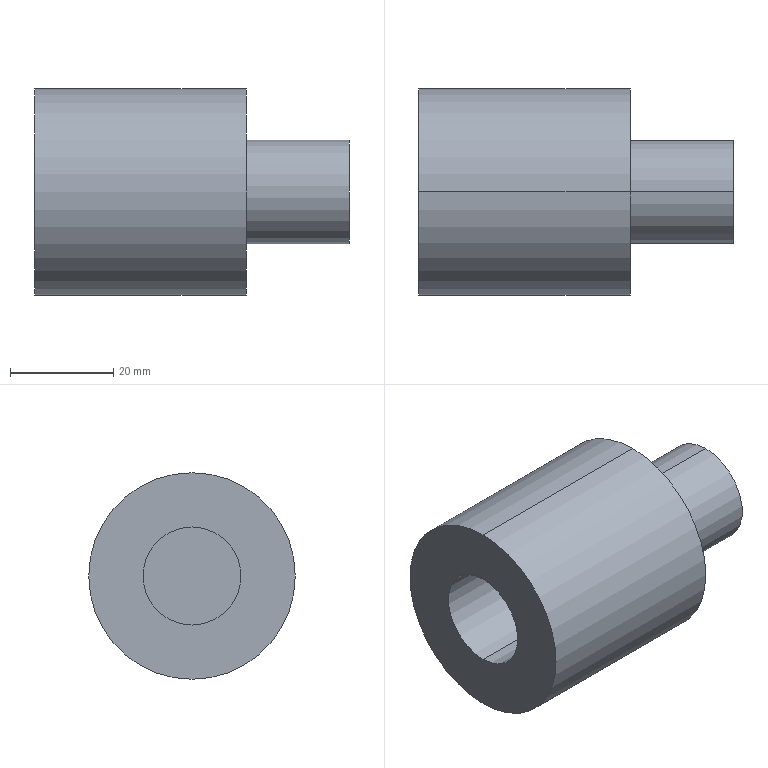Part | STEP file | _MAX100010001NA0_cupling2 | 1 solid | 10 faces | box 61 x 40 x 40 mm | volume 52985 mm3 | cylinder 6 | plane 4 | commonest cylinder face diameters 19 x2 20 x2 40 x2
STEP:
#1=CARTESIAN_POINT('',(504.,0.,20.));
#2=VERTEX_POINT('',#1);
#3=CARTESIAN_POINT('',(504.,0.,-20.));
#4=VERTEX_POINT('',#3);
#5=CARTESIAN_POINT('',(504.,0.,0.));
#6=DIRECTION('',(-1.,0.,0.));
#7=DIRECTION('',(0.,0.,1.));
#8=AXIS2_PLACEMENT_3D('',#5,#6,#7);
#9=CIRCLE('',#8,20.);
#10=EDGE_CURVE('',#2,#4,#9,.T.);
#11=ORIENTED_EDGE('',*,*,#10,.T.);
#12=CARTESIAN_POINT('',(463.,0.,-20.));
#13=VERTEX_POINT('',#12);
#14=CARTESIAN_POINT('',(524.,0.,-20.));
#15=DIRECTION('',(-1.,0.,0.));
#16=VECTOR('',#15,1000.);
#17=LINE('',#14,#16);
#18=EDGE_CURVE('',#4,#13,#17,.T.);
#19=ORIENTED_EDGE('',*,*,#18,.T.);
#20=CARTESIAN_POINT('',(463.,0.,20.));
#21=VERTEX_POINT('',#20);
#22=CARTESIAN_POINT('',(463.,0.,0.));
#23=DIRECTION('',(1.,0.,0.));
#24=DIRECTION('',(0.,0.,1.));
#25=AXIS2_PLACEMENT_3D('',#22,#23,#24);
#26=CIRCLE('',#25,20.);
#27=EDGE_CURVE('',#13,#21,#26,.T.);
#28=ORIENTED_EDGE('',*,*,#27,.T.);
#29=CARTESIAN_POINT('',(524.,0.,20.));
#30=DIRECTION('',(-1.,0.,0.));
#31=VECTOR('',#30,1000.);
#32=LINE('',#29,#31);
#33=EDGE_CURVE('',#2,#21,#32,.T.);
#34=ORIENTED_EDGE('',*,*,#33,.F.);
#35=EDGE_LOOP('',(#11,#19,#28,#34));
#36=FACE_OUTER_BOUND('',#35,.T.);
#37=CARTESIAN_POINT('',(524.,0.,0.));
#38=DIRECTION('',(-1.,0.,0.));
#39=DIRECTION('',(0.,0.,1.));
#40=AXIS2_PLACEMENT_3D('',#37,#38,#39);
#41=CYLINDRICAL_SURFACE('',#40,20.);
#42=ADVANCED_FACE('',(#36),#41,.T.);
#43=CARTESIAN_POINT('',(480.,0.,-9.5));
#44=VERTEX_POINT('',#43);
#45=CARTESIAN_POINT('',(480.,0.,9.5));
#46=VERTEX_POINT('',#45);
#47=CARTESIAN_POINT('',(480.,0.,0.));
#48=DIRECTION('',(-1.,0.,0.));
#49=DIRECTION('',(0.,0.,1.));
#50=AXIS2_PLACEMENT_3D('',#47,#48,#49);
#51=CIRCLE('',#50,9.5);
#52=EDGE_CURVE('',#44,#46,#51,.T.);
#53=ORIENTED_EDGE('',*,*,#52,.F.);
#54=CARTESIAN_POINT('',(463.,0.,-9.5));
#55=VERTEX_POINT('',#54);
#56=CARTESIAN_POINT('',(524.,0.,-9.5));
#57=DIRECTION('',(-1.,0.,0.));
#58=VECTOR('',#57,1000.);
#59=LINE('',#56,#58);
#60=EDGE_CURVE('',#44,#55,#59,.T.);
#61=ORIENTED_EDGE('',*,*,#60,.T.);
#62=CARTESIAN_POINT('',(463.,0.,9.5));
#63=VERTEX_POINT('',#62);
#64=CARTESIAN_POINT('',(463.,0.,0.));
#65=DIRECTION('',(-1.,0.,0.));
#66=DIRECTION('',(0.,0.,1.));
#67=AXIS2_PLACEMENT_3D('',#64,#65,#66);
#68=CIRCLE('',#67,9.5);
#69=EDGE_CURVE('',#55,#63,#68,.T.);
#70=ORIENTED_EDGE('',*,*,#69,.T.);
#71=CARTESIAN_POINT('',(524.,0.,9.5));
#72=DIRECTION('',(-1.,0.,0.));
#73=VECTOR('',#72,1000.);
#74=LINE('',#71,#73);
#75=EDGE_CURVE('',#46,#63,#74,.T.);
#76=ORIENTED_EDGE('',*,*,#75,.F.);
#77=EDGE_LOOP('',(#53,#61,#70,#76));
#78=FACE_OUTER_BOUND('',#77,.T.);
#79=CARTESIAN_POINT('',(524.,0.,0.));
#80=DIRECTION('',(-1.,0.,0.));
#81=DIRECTION('',(0.,0.,1.));
#82=AXIS2_PLACEMENT_3D('',#79,#80,#81);
#83=CYLINDRICAL_SURFACE('',#82,9.5);
#84=ADVANCED_FACE('',(#78),#83,.F.);
#85=CARTESIAN_POINT('',(524.,0.,10.));
#86=VERTEX_POINT('',#85);
#87=CARTESIAN_POINT('',(524.,0.,-10.));
#88=VERTEX_POINT('',#87);
#89=CARTESIAN_POINT('',(524.,0.,0.));
#90=DIRECTION('',(-1.,0.,0.));
#91=DIRECTION('',(0.,0.,1.));
#92=AXIS2_PLACEMENT_3D('',#89,#90,#91);
#93=CIRCLE('',#92,10.);
#94=EDGE_CURVE('',#86,#88,#93,.T.);
#95=ORIENTED_EDGE('',*,*,#94,.T.);
#96=CARTESIAN_POINT('',(504.,0.,-10.));
#97=VERTEX_POINT('',#96);
#98=CARTESIAN_POINT('',(524.,0.,-10.));
#99=DIRECTION('',(-1.,0.,0.));
#100=VECTOR('',#99,1000.);
#101=LINE('',#98,#100);
#102=EDGE_CURVE('',#88,#97,#101,.T.);
#103=ORIENTED_EDGE('',*,*,#102,.T.);
#104=CARTESIAN_POINT('',(504.,0.,10.));
#105=VERTEX_POINT('',#104);
#106=CARTESIAN_POINT('',(504.,0.,0.));
#107=DIRECTION('',(1.,0.,0.));
#108=DIRECTION('',(0.,0.,1.));
#109=AXIS2_PLACEMENT_3D('',#106,#107,#108);
#110=CIRCLE('',#109,10.);
#111=EDGE_CURVE('',#97,#105,#110,.T.);
#112=ORIENTED_EDGE('',*,*,#111,.T.);
#113=CARTESIAN_POINT('',(524.,0.,10.));
#114=DIRECTION('',(-1.,0.,0.));
#115=VECTOR('',#114,1000.);
#116=LINE('',#113,#115);
#117=EDGE_CURVE('',#86,#105,#116,.T.);
#118=ORIENTED_EDGE('',*,*,#117,.F.);
#119=EDGE_LOOP('',(#95,#103,#112,#118));
#120=FACE_OUTER_BOUND('',#119,.T.);
#121=CARTESIAN_POINT('',(524.,0.,0.));
#122=DIRECTION('',(-1.,0.,0.));
#123=DIRECTION('',(0.,0.,1.));
#124=AXIS2_PLACEMENT_3D('',#121,#122,#123);
#125=CYLINDRICAL_SURFACE('',#124,10.);
#126=ADVANCED_FACE('',(#120),#125,.T.);
#127=ORIENTED_EDGE('',*,*,#18,.F.);
#128=CARTESIAN_POINT('',(504.,0.,0.));
#129=DIRECTION('',(-1.,0.,0.));
#130=DIRECTION('',(0.,0.,1.));
#131=AXIS2_PLACEMENT_3D('',#128,#129,#130);
#132=CIRCLE('',#131,20.);
#133=EDGE_CURVE('',#4,#2,#132,.T.);
#134=ORIENTED_EDGE('',*,*,#133,.T.);
#135=ORIENTED_EDGE('',*,*,#33,.T.);
#136=CARTESIAN_POINT('',(463.,0.,0.));
#137=DIRECTION('',(1.,0.,0.));
#138=DIRECTION('',(0.,0.,1.));
#139=AXIS2_PLACEMENT_3D('',#136,#137,#138);
#140=CIRCLE('',#139,20.);
#141=EDGE_CURVE('',#21,#13,#140,.T.);
#142=ORIENTED_EDGE('',*,*,#141,.T.);
#143=EDGE_LOOP('',(#127,#134,#135,#142));
#144=FACE_OUTER_BOUND('',#143,.T.);
#145=CARTESIAN_POINT('',(524.,0.,0.));
#146=DIRECTION('',(-1.,0.,0.));
#147=DIRECTION('',(0.,0.,1.));
#148=AXIS2_PLACEMENT_3D('',#145,#146,#147);
#149=CYLINDRICAL_SURFACE('',#148,20.);
#150=ADVANCED_FACE('',(#144),#149,.T.);
#151=CARTESIAN_POINT('',(463.,0.,0.));
#152=DIRECTION('',(-1.,0.,0.));
#153=DIRECTION('',(0.,0.,1.));
#154=AXIS2_PLACEMENT_3D('',#151,#152,#153);
#155=CIRCLE('',#154,9.5);
#156=EDGE_CURVE('',#63,#55,#155,.T.);
#157=ORIENTED_EDGE('',*,*,#156,.F.);
#158=ORIENTED_EDGE('',*,*,#69,.F.);
#159=EDGE_LOOP('',(#157,#158));
#160=FACE_BOUND('',#159,.T.);
#161=ORIENTED_EDGE('',*,*,#141,.F.);
#162=ORIENTED_EDGE('',*,*,#27,.F.);
#163=EDGE_LOOP('',(#161,#162));
#164=FACE_OUTER_BOUND('',#163,.T.);
#165=CARTESIAN_POINT('',(463.,9.5,0.));
#166=DIRECTION('',(1.,0.,0.));
#167=DIRECTION('',(0.,0.,-1.));
#168=AXIS2_PLACEMENT_3D('',#165,#166,#167);
#169=PLANE('',#168);
#170=ADVANCED_FACE('',(#160,#164),#169,.F.);
#171=ORIENTED_EDGE('',*,*,#10,.F.);
#172=ORIENTED_EDGE('',*,*,#133,.F.);
#173=EDGE_LOOP('',(#171,#172));
#174=FACE_OUTER_BOUND('',#173,.T.);
#175=CARTESIAN_POINT('',(504.,0.,0.));
#176=DIRECTION('',(1.,0.,0.));
#177=DIRECTION('',(0.,0.,1.));
#178=AXIS2_PLACEMENT_3D('',#175,#176,#177);
#179=CIRCLE('',#178,10.);
#180=EDGE_CURVE('',#105,#97,#179,.T.);
#181=ORIENTED_EDGE('',*,*,#180,.F.);
#182=ORIENTED_EDGE('',*,*,#111,.F.);
#183=EDGE_LOOP('',(#181,#182));
#184=FACE_BOUND('',#183,.T.);
#185=CARTESIAN_POINT('',(504.,20.,0.));
#186=DIRECTION('',(-1.,0.,0.));
#187=DIRECTION('',(0.,0.,1.));
#188=AXIS2_PLACEMENT_3D('',#185,#186,#187);
#189=PLANE('',#188);
#190=ADVANCED_FACE('',(#174,#184),#189,.F.);
#191=ORIENTED_EDGE('',*,*,#60,.F.);
#192=CARTESIAN_POINT('',(480.,0.,0.));
#193=DIRECTION('',(-1.,0.,0.));
#194=DIRECTION('',(0.,0.,1.));
#195=AXIS2_PLACEMENT_3D('',#192,#193,#194);
#196=CIRCLE('',#195,9.5);
#197=EDGE_CURVE('',#46,#44,#196,.T.);
#198=ORIENTED_EDGE('',*,*,#197,.F.);
#199=ORIENTED_EDGE('',*,*,#75,.T.);
#200=ORIENTED_EDGE('',*,*,#156,.T.);
#201=EDGE_LOOP('',(#191,#198,#199,#200));
#202=FACE_OUTER_BOUND('',#201,.T.);
#203=CARTESIAN_POINT('',(524.,0.,0.));
#204=DIRECTION('',(-1.,0.,0.));
#205=DIRECTION('',(0.,0.,1.));
#206=AXIS2_PLACEMENT_3D('',#203,#204,#205);
#207=CYLINDRICAL_SURFACE('',#206,9.5);
#208=ADVANCED_FACE('',(#202),#207,.F.);
#209=ORIENTED_EDGE('',*,*,#102,.F.);
#210=CARTESIAN_POINT('',(524.,0.,0.));
#211=DIRECTION('',(-1.,0.,0.));
#212=DIRECTION('',(0.,0.,1.));
#213=AXIS2_PLACEMENT_3D('',#210,#211,#212);
#214=CIRCLE('',#213,10.);
#215=EDGE_CURVE('',#88,#86,#214,.T.);
#216=ORIENTED_EDGE('',*,*,#215,.T.);
#217=ORIENTED_EDGE('',*,*,#117,.T.);
#218=ORIENTED_EDGE('',*,*,#180,.T.);
#219=EDGE_LOOP('',(#209,#216,#217,#218));
#220=FACE_OUTER_BOUND('',#219,.T.);
#221=CARTESIAN_POINT('',(524.,0.,0.));
#222=DIRECTION('',(-1.,0.,0.));
#223=DIRECTION('',(0.,0.,1.));
#224=AXIS2_PLACEMENT_3D('',#221,#222,#223);
#225=CYLINDRICAL_SURFACE('',#224,10.);
#226=ADVANCED_FACE('',(#220),#225,.T.);
#227=ORIENTED_EDGE('',*,*,#197,.T.);
#228=ORIENTED_EDGE('',*,*,#52,.T.);
#229=EDGE_LOOP('',(#227,#228));
#230=FACE_OUTER_BOUND('',#229,.T.);
#231=CARTESIAN_POINT('',(480.,0.,0.));
#232=DIRECTION('',(1.,0.,0.));
#233=DIRECTION('',(0.,0.,-1.));
#234=AXIS2_PLACEMENT_3D('',#231,#232,#233);
#235=PLANE('',#234);
#236=ADVANCED_FACE('',(#230),#235,.F.);
#237=ORIENTED_EDGE('',*,*,#94,.F.);
#238=ORIENTED_EDGE('',*,*,#215,.F.);
#239=EDGE_LOOP('',(#237,#238));
#240=FACE_OUTER_BOUND('',#239,.T.);
#241=CARTESIAN_POINT('',(524.,10.,0.));
#242=DIRECTION('',(-1.,0.,0.));
#243=DIRECTION('',(0.,0.,1.));
#244=AXIS2_PLACEMENT_3D('',#241,#242,#243);
#245=PLANE('',#244);
#246=ADVANCED_FACE('',(#240),#245,.F.);
#247=CLOSED_SHELL('',(#42,#84,#126,#150,#170,#190,#208,#226,#236,#246));
#248=MANIFOLD_SOLID_BREP('',#247);
#249=CARTESIAN_POINT('',(0.,0.,0.));
#250=DIRECTION('',(0.,0.,1.));
#251=DIRECTION('',(1.,0.,0.));
#252=AXIS2_PLACEMENT_3D('',#249,#250,#251);
#253=(LENGTH_UNIT()NAMED_UNIT(*)SI_UNIT(.MILLI.,.METRE.));
#254=UNCERTAINTY_MEASURE_WITH_UNIT(LENGTH_MEASURE(0.00001),#253,'','');
#255=(NAMED_UNIT(*)PLANE_ANGLE_UNIT()SI_UNIT($,.RADIAN.));
#256=(NAMED_UNIT(*)SI_UNIT($,.STERADIAN.)SOLID_ANGLE_UNIT());
#257=(GEOMETRIC_REPRESENTATION_CONTEXT(3)GLOBAL_UNCERTAINTY_ASSIGNED_CONTEXT((#254))GLOBAL_UNIT_ASSIGNED_CONTEXT((#253,#255,#256))REPRESENTATION_CONTEXT('',''));
#258=ADVANCED_BREP_SHAPE_REPRESENTATION('',(#248,#252),#257);